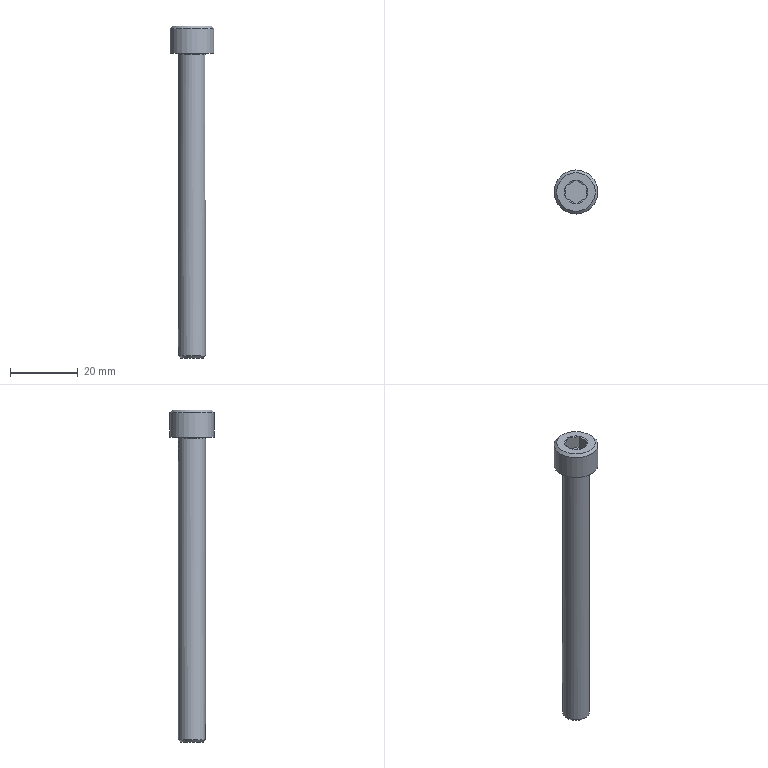Part | STEP file | solid 202 | 1 solid | 106 faces | box 13 x 13 x 98 mm | volume 5444 mm3 | plane 53 | other 36 | cylinder 8 | sphere 6 | cone 2 | torus 1 | commonest cylinder face diameters 8 x7 13 x1